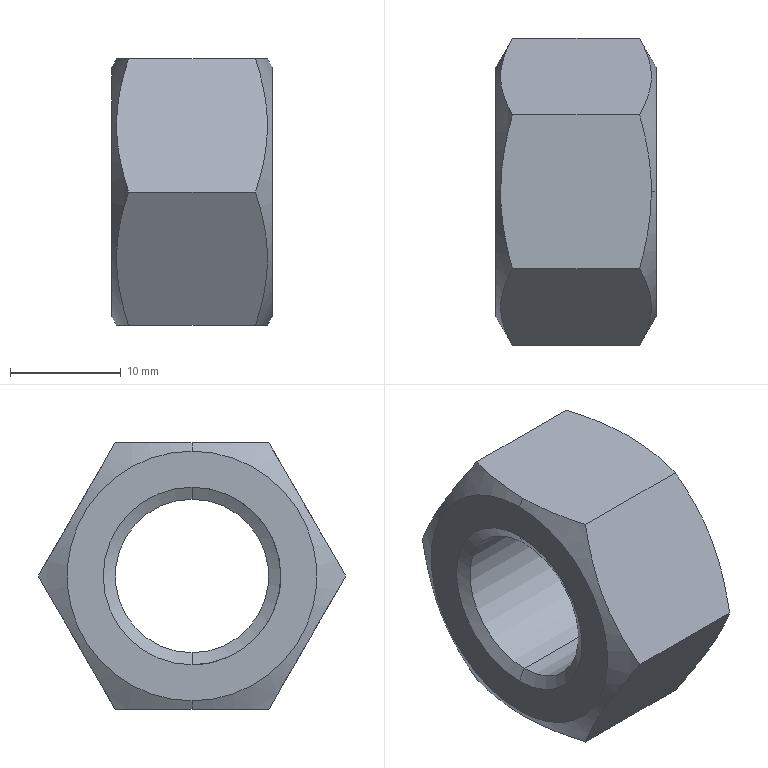Part | STEP file | Positioning_id1818_x_t | 1 solid | 23 faces | box 14.45 x 27.713 x 24 mm | volume 4910 mm3 | plane 9 | cone 8 | cylinder 6 | commonest cylinder face diameters 13.835 x2 16 x2 16.001 x2